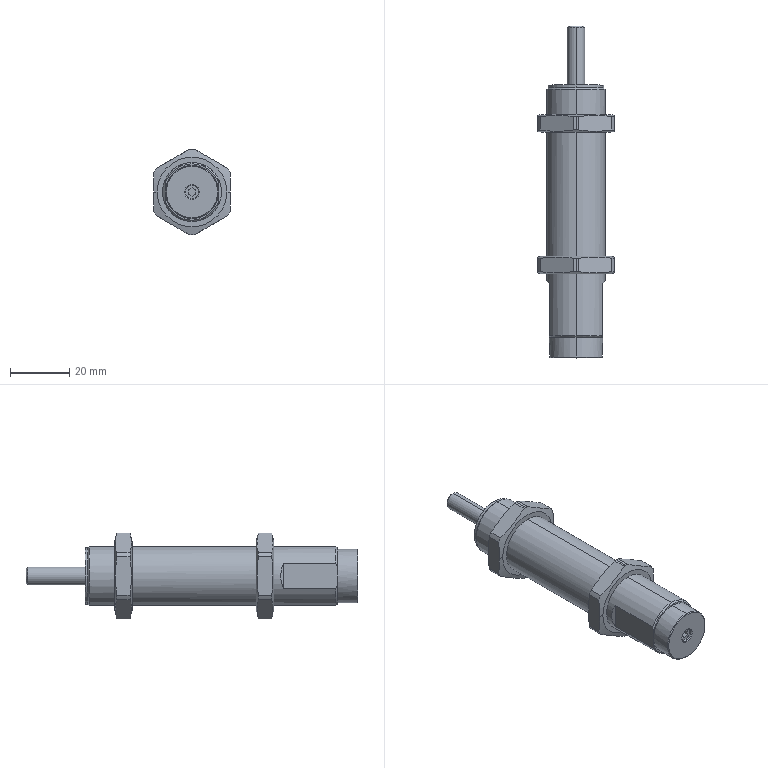Part | SolidWorks | features BaseBody 3 | 3 solids | 91 faces | box 26 x 112.5 x 29.132 mm | volume 32268 mm3 | plane 34 | cone 29 | cylinder 28 | commonest cylinder face diameters 29.132 x14 19.188 x4 4.459 x2 6 x2 18 x2 19 x2